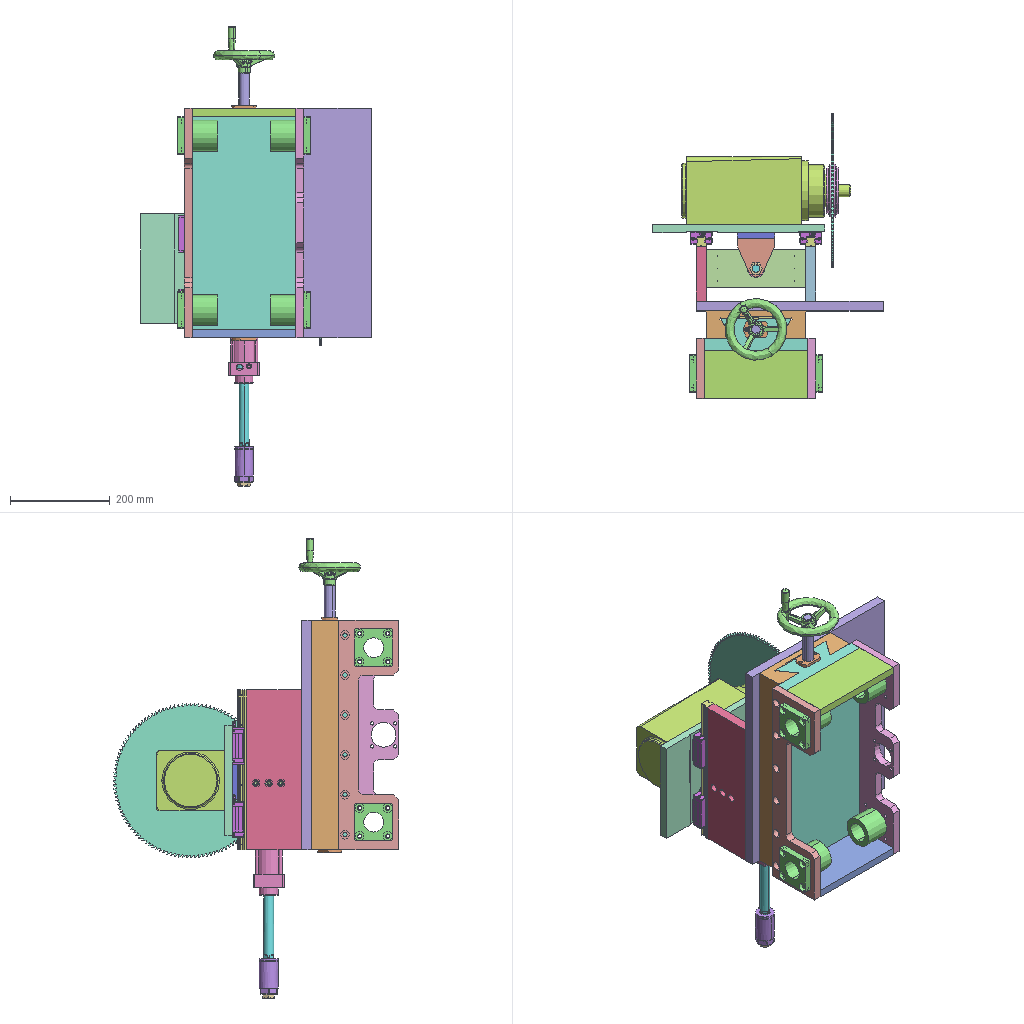Assembly | SolidWorks | 30 different items | 44 placed | box 462 x 572 x 923 mm
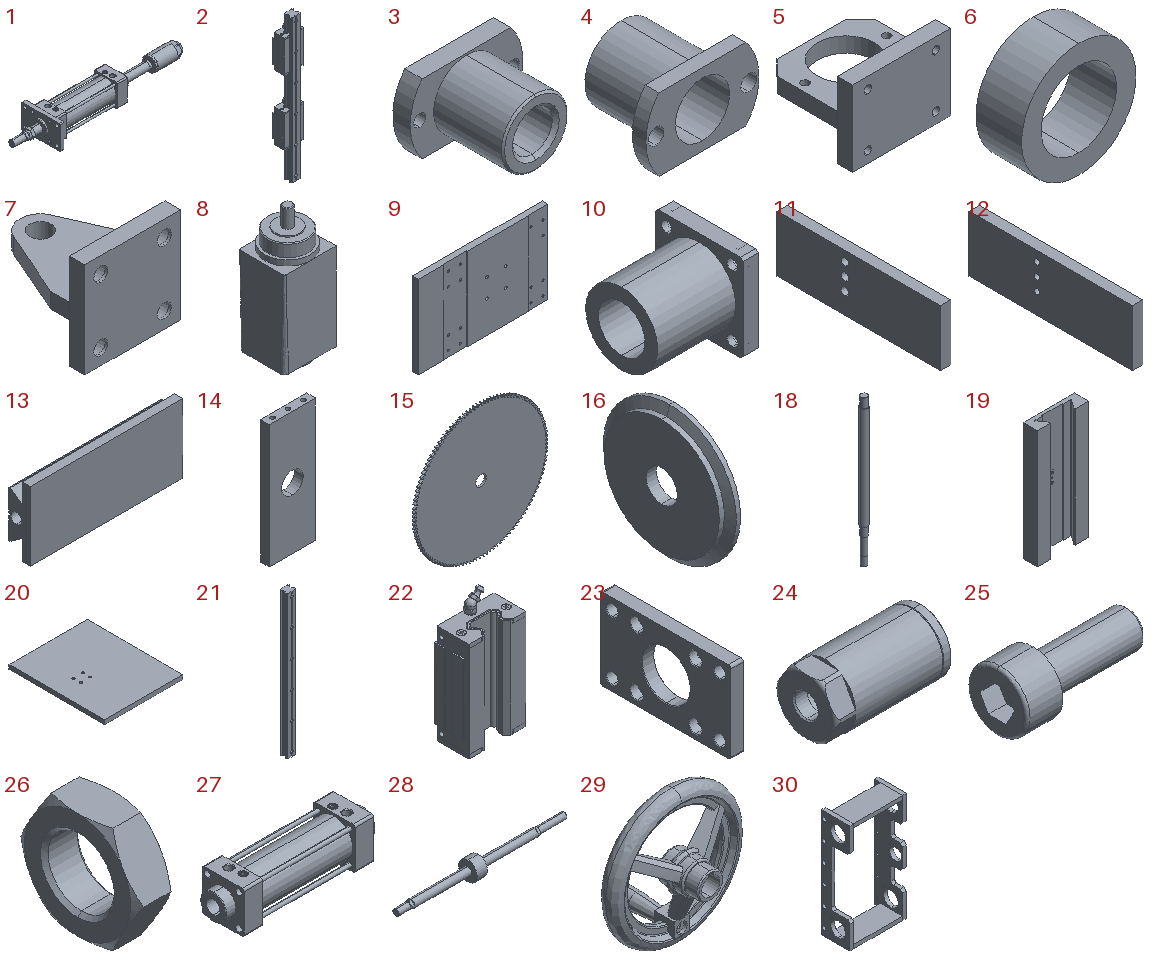Parts list (item | name | quantity | parent item | size | volume | features):
1 | (subassembly) | x1 | - | 452 x 104 x 65 mm | 566807 mm3 | features CompositeCurve 1
2 | (subassembly) | x2 | - | 44 x 29.99 x 320 mm | 212092 mm3 | -
3 | - | x1 | - | 65 x 50 x 40 mm | 47707 mm3 | features ICE 4, Chamfer 2, CirPattern 1, Extrusion 1
4 | - | x2 | - | 50 x 36 x 32 mm | 16277 mm3 | features ICE 2, Revolution 1
5 | - | x1 | - | 65 x 60 x 50 mm | 51481 mm3 | features HoleWzd 2, ICE 2, Chamfer 1, Extrusion 1
6 | - | x1 | - | 25 x 10 x 25 mm | 2770 mm3 | features Extrusion 1
7 | - | x1 | - | 75 x 88.5 x 75 mm | 103360 mm3 | features ICE 3, Extrusion 1, HoleWzd 1
8 | - | x1 | - | 136 x 120 x 339 mm | 4326420 mm3 | features ICE 5, Chamfer 3, Extrusion 1, Fillet 1, VarFillet 1
9 | - | x1 | - | 345 x 16 x 220 mm | 1151722 mm3 | features HoleWzd 2, Extrusion 1, ICE 1
10 | - | x4 | - | 80 x 75 x 75 mm | 165352 mm3 | features Chamfer 1, Extrusion 1, HoleWzd 1, ICE 1
11 | - | x1 | - | 20 x 320 x 110 mm | 695848 mm3 | features Extrusion 1, HoleWzd 1
12 | - | x1 | - | 20 x 320 x 110 mm | 695848 mm3 | features Extrusion 1, HoleWzd 1
13 | - | x1 | - | 460 x 65 x 208 mm | 2873853 mm3 | features HoleWzd 2, ICE 2, Extrusion 1
14 | - | x1 | - | 75 x 14 x 200 mm | 191534 mm3 | features HoleWzd 2, Extrusion 1, ICE 1
15 | - | x1 | - | 309.988 x 5 x 309.988 mm | 361074 mm3 | features Extrusion 1, ICE 1
16 | - | x2 | - | 10 x 106 x 106 mm | 67420 mm3 | features Revolution 1
17 | - | x1 | - | - | - | -
18 | - | x1 | - | 28 x 28 x 572 mm | 313729 mm3 | features Chamfer 4, ICE 4, Extrusion 1
19 | - | x1 | - | 200 x 55 x 460 mm | 2781667 mm3 | features HoleWzd 2, Extrusion 1
20 | - | x1 | - | 375 x 460 x 20 mm | 3445803 mm3 | features Extrusion 1, HoleWzd 1
21 | - | x2 | in 2 | 20 x 18 x 320 mm | 90311 mm3 | features ICE 9, Chamfer 3, Fillet 3, HoleWzd 2, Extrusion 1
22 | - | x4 | in 2 | 44 x 25 x 86.312 mm | 60891 mm3 | features ICE 34, HoleWzd 8, Chamfer 4, BaseBody 1
23 | - | x1 | in 1 | 10 x 104 x 65 mm | 50722 mm3 | features RefAxis 15, 3DProfileFeature 5, RevCut 3, LPattern 2, Extrusion 1
24 | - | x1 | in 1 | 71 x 38 x 38 mm | 56473 mm3 | features RefAxis 3, 3DProfileFeature 1, ICE 1, RevCut 1, Revolution 1
25 | - | x4 | in 1 | 22 x 10 x 10 mm | 853.723 mm3 | features RefAxis 3, 3DProfileFeature 1, ICE 1, Revolution 1
26 | - | x2 | in 1 | 8 x 26.558 x 23 mm | 2309 mm3 | features RefAxis 3, 3DProfileFeature 1, ICE 1, RevCut 1, Revolution 1
27 | - | x1 | in 1 | 223 x 62 x 62 mm | 281085 mm3 | features RefAxis 48, 3DProfileFeature 16, RevCut 7, LPattern 3, Revolution 3, ICE 2, Extrusion 1
28 | - | x1 | in 1 | 444 x 49.5 x 49.5 mm | 170493 mm3 | features RefAxis 15, 3DProfileFeature 5, ICE 4, Revolution 2
29 | - | x1 | - | 124 x 95 x 124 mm | 109982 mm3 | features Draft 7, ICE 5, Fillet 4, BaseBody 1, Chamfer 1, HoleWzd 1, RevCut 1
30 | - | x1 | - | 240 x 120 x 460 mm | 1705402 mm3 | features ICE 7, HoleWzd 3, Chamfer 2, Fillet 2, MirrorPattern 2, Extrusion 1
Mates (type | each side: item.copy, entity, surface, feature):
In the top assembly
Coincident | 30.1 face plane Boss-Extrude2 | 13.1 face plane Boss-Extrude1
Coincident | 30.1 face plane Boss-Extrude1 | 13.1 face plane Boss-Extrude1 | 2 times
InPlace | 13.1 face plane Boss-Extrude1 | 19.1 plane
InPlace | 19.1 face plane Boss-Extrude1 | 20.1 plane
Concentric | 30.1 face cylinder Cut-Extrude2 | 10.1 face cylinder Boss-Extrude1
Coincident | 30.1 face plane Boss-Extrude1 | 10.1 face plane Boss-Extrude2
Parallel | 10.1 face plane Boss-Extrude2 | 30.1 face plane Boss-Extrude1
InPlace | 20.1 face plane Boss-Extrude1 | 11.1 plane
InPlace | 20.1 face plane Boss-Extrude1 | 12.1 plane
Coincident | 11.1 face plane Boss-Extrude1 | 21.1 face plane Boss-Extrude1 | 2 times
Width | 21.1 face plane Boss-Extrude1 | 21.1 face plane Boss-Extrude1 | 11.1 face plane Boss-Extrude1 | 11.1 face plane Boss-Extrude1
Coincident | 12.1 face plane Boss-Extrude1 | 21.2 face plane Boss-Extrude1 | 2 times
Width | 21.2 face plane Boss-Extrude1 | 21.2 face plane Boss-Extrude1 | 12.1 face plane Boss-Extrude1 | 12.1 face plane Boss-Extrude1
Coincident | 22.1 face plane Boss-Extrude13 | 9.1 face plane Cut-Extrude1
Concentric | 22.1 face cylinder Ø5.0 (5) Diameter Hole1 | 9.1 face cylinder CBORE for M5 Hex Head Bolt1
Concentric | 22.2 face cylinder Ø5.0 (5) Diameter Hole1 | 9.1 face cylinder CBORE for M5 Hex Head Bolt1
Coincident | 22.1 face plane Boss-Extrude2 | 22.3 face plane Boss-Extrude2
Coincident | 22.2 face plane Boss-Extrude9 | 22.4 face plane Boss-Extrude9
Coincident | 9.1 face plane Boss-Extrude1 | 7.1 face plane Boss-Extrude1
Width | 7.1 face plane Boss-Extrude1 | 7.1 face plane Boss-Extrude1 | 11.1 face plane Boss-Extrude1 | 12.1 face plane Boss-Extrude1
Width | 7.1 face plane Boss-Extrude1 | 7.1 face plane Boss-Extrude1 | 9.1 face plane Boss-Extrude1 | 9.1 face plane Boss-Extrude1
InPlace | 12.1 face plane Boss-Extrude1 | 14.1 plane
Concentric | 14.1 face cylinder Cut-Extrude1 | 27.1 face cylinder Revolve3
Coincident | 14.1 face plane Boss-Extrude1 | 23.1 face plane Boss-Extrude1
Parallel | 14.1 face plane Boss-Extrude1 | 23.1 face plane Boss-Extrude1
Concentric | 28.1 face cylinder Revolve1 | 6.1 face cylinder Boss-Extrude1
Coincident | 28.1 edge | 6.1 face plane Boss-Extrude1
Coincident | 7.1 face plane Boss-Extrude2 | 6.1 face plane Boss-Extrude1
Concentric | 7.1 face cylinder Cut-Extrude1 | 26.1 face cylinder Cut-Revolve1
Coincident | 7.1 face plane Boss-Extrude2 | 26.1 face plane Revolve1
Coincident | 9.1 face plane Boss-Extrude1 | 8.1 face plane Boss-Extrude1
Width | 8.1 face plane Boss-Extrude1 | 8.1 face plane Boss-Extrude1 | 9.1 face plane Boss-Extrude1 | 9.1 face plane Boss-Extrude1
Coincident | 9.1 face plane Boss-Extrude1 | 8.1 face plane Boss-Extrude3
Concentric | 8.1 face cylinder Boss-Extrude5 | 16.1 face cylinder Revolve1
Coincident | 8.1 face plane Boss-Extrude4 | 16.1 face plane Revolve1
Concentric | 8.1 face cylinder Boss-Extrude5 | 15.1 face cylinder Boss-Extrude1
Coincident | 16.1 face plane Revolve1 | 15.1 face plane Boss-Extrude1
Concentric | 8.1 face cylinder Boss-Extrude5 | 16.2 face cylinder Revolve1
Coincident | 15.1 face plane Boss-Extrude1 | 16.2 face plane Revolve1
Concentric | 13.1 face cylinder Cut-Extrude2 | 4.1 face cylinder Revolve1
Coincident | 13.1 face plane Boss-Extrude1 | 4.1 face plane Revolve1
Concentric | 13.1 face cylinder Cut-Extrude2 | 4.2 face cylinder Revolve1
Coincident | 13.1 face plane Boss-Extrude1 | 4.2 face plane Revolve1
InPlace | 4.2 face plane Revolve1 | 18.1 plane
Concentric | 18.1 face cylinder Cut-Extrude1 | 29.1 face cylinder Cut-Extrude1
Coincident | 18.1 face plane Cut-Extrude1 | 29.1 face plane Boss-Extrude4
Parallel | 18.1 face plane Cut-Extrude2 | 29.1 face plane Cut-Extrude1
Concentric | 18.1 face cylinder Boss-Extrude3 | 3.1 face cylinder Cut-Extrude1
Parallel | 13.1 face plane Cut-Extrude1 | 3.1 face plane Cut-Extrude3
Concentric | 3.1 face cylinder Boss-Extrude1 | 5.1 face cylinder Cut-Extrude1
Coincident | 3.1 face plane Boss-Extrude2 | 5.1 face plane Boss-Extrude2
Parallel | 20.1 face plane Boss-Extrude1 | 5.1 face plane Boss-Extrude1
Width | 20.1 face plane Boss-Extrude1 | 20.1 face plane Boss-Extrude1 | 5.1 face plane Boss-Extrude1 | 5.1 face plane Boss-Extrude1
In subassembly 2
Coincident | 21.3 face plane Boss-Extrude1 | 22.5 face plane Cut-Extrude11
Width | 22.5 face plane Boss-Extrude11 | 22.5 face plane Boss-Extrude12 | 21.3 face plane Boss-Extrude1 | 21.3 face plane Boss-Extrude1
Coincident | 21.3 face plane Boss-Extrude1 | 22.6 face plane Cut-Extrude11
Width | 22.6 face plane Boss-Extrude11 | 22.6 face plane Boss-Extrude12 | 21.3 face plane Boss-Extrude1 | 21.3 face plane Boss-Extrude1
In subassembly 1
Coincident | 27.2 axis | 28.2 axis
PlanarAngleDim | 28.2 plane | 27.2 plane
Coincident | 28.2 axis | 26.2 axis
PlanarAngleDim | 26.2 plane | 28.2 plane
Coincident | 28.2 axis | 24.1 axis
PlanarAngleDim | 24.1 plane | 28.2 plane
Coincident | 28.2 axis | 26.3 axis
PlanarAngleDim | 26.3 plane | 28.2 plane
Coincident | 27.2 axis | 23.2 axis
PlanarAngleDim | 23.2 plane | 27.2 plane
Coincident | 23.2 axis | 25.1 axis
PlanarAngleDim | 25.1 plane | 23.2 plane
Coincident | 23.2 axis | 25.2 axis
PlanarAngleDim | 25.2 plane | 23.2 plane
Coincident | 23.2 axis | 25.3 axis
PlanarAngleDim | 25.3 plane | 23.2 plane
Coincident | 23.2 axis | 25.4 axis
PlanarAngleDim | 25.4 plane | 23.2 plane
Coincident | 27.2 face plane Boss-Extrude1 | 23.2 face plane Boss-Extrude1
Coincident | 28.2 edge | 24.1 face plane Revolve1
Coincident | 24.1 face plane Revolve1 | 26.3 face plane Revolve1
Concentric | 24.1 face cylinder Revolve1 | 26.3 face cylinder Cut-Revolve1